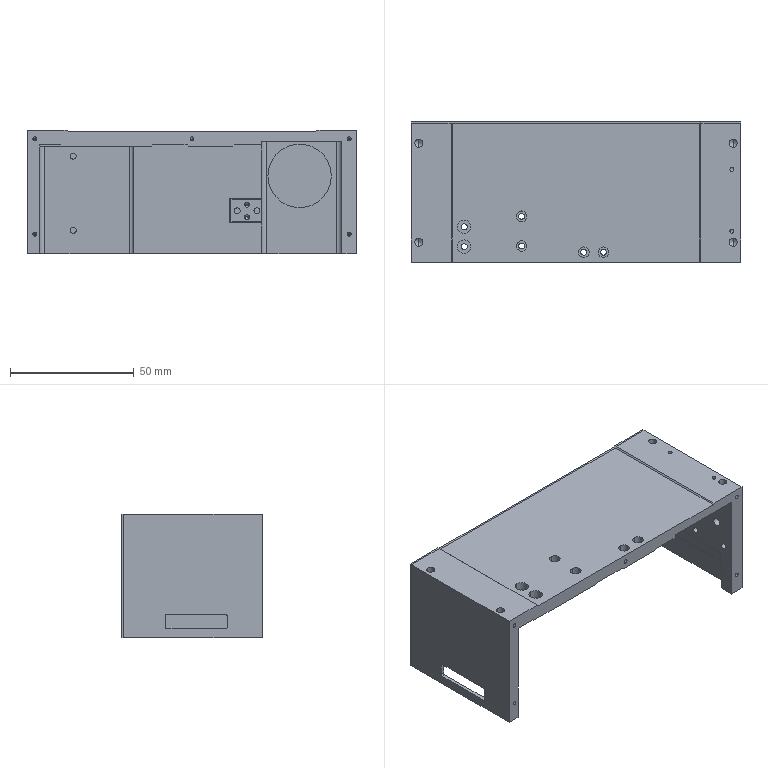NC program | NX | posted with a generic post | part box 133 x 56.74 x 50 mm
Whole program:
N10 G17 G21 G94 G90
(FLOOR_WALL_1_COPY , TOOL : D10)
N12 T10 M6
N14 G54
N16 G17 G0 G90 X22.033 Y-33. B0. C0. S9500 M3
N18 G43 Z30. H10
N20 Z2.685
N22 G94 G1 Z-0.315 F1000.
N24 Y-30.
N26 X-71.5 F2500.
N28 Y30.
N30 X-48.429
N32 X-47.929 Y29.5
N34 X47.929
N36 X48.429 Y30.
N38 X71.5
N40 Y-30.
N42 X22.033
N44 Y-25.
N46 X-66.5
N48 Y25.
N50 X-54.649
N52 G3 X-45.371 Y-15.019 R21.6
N54 G1 X-45.804 Y-20.
N56 X-61.5
N58 Y-13.085
N60 G3 X-45.804 Y-20. R26.6
N62 G1 X-45.371 Y-15.019
N64 G3 X-31.56 Y24.5 R21.6
N66 G1 X-32.113 Y23.667
N68 G2 X-26.333 Y-4.887 R20.6
N70 X-32.113 Y23.667 R-20.6
N72 G1 X-31.56 Y24.5
N74 X47.929
N76 G3 X50.108 Y25. R5.
N78 G1 X66.5
N80 Y-25.
N82 X22.033
N84 Y-20.
N86 X-41.196
N88 G3 X-20.293 Y19.5 R26.6
N90 G1 X47.929
N92 G3 X51.051 Y20. R10.
N94 G1 X61.5
N96 Y-20.
N98 X22.033
N100 Y-15.
N102 X-20.342
N104 G3 X-12.929 Y14.5 R31.6
N106 G1 X47.929
N108 G3 X51.77 Y15. R15.
N110 G1 X56.5
N112 Y-15.
N114 X22.033
N116 Y-10.
N118 X-10.83
N120 G3 X-7.023 Y9.5 R36.6
N122 G1 X47.929
N124 G3 X51.5 Y9.821 R20.
N126 G1 Y-10.
N128 X22.033
N130 Y-5.
N132 X-3.521
N134 G3 X-1.948 Y4.5 R41.6
N136 G1 X46.5
N138 Y-5.
N140 X22.033
N142 Y-0.5
N144 X2.065
N146 G3 X2.139 Y0. R46.1
N148 G1 X42.
N150 Y-0.5
N152 X22.033
N154 Y-3.5
N156 Z2.685
N158 G0 Z30.
N160 Y-33.
N162 Z2.36
N164 G1 Z-0.64 F1000.
N166 Y-30.
N168 X-71.5 F2500.
N170 Y30.
N172 X-48.429
N174 X-47.929 Y29.5
N176 X47.929
N178 X48.429 Y30.
N180 X71.5
N182 Y-30.
N184 X22.033
N186 Y-25.
N188 X-66.5
N190 Y25.
N192 X-54.649
N194 G3 X-45.371 Y-15.019 R21.6
N196 G1 X-45.804 Y-20.
N198 X-61.5
N200 Y-13.085
N202 G3 X-45.804 Y-20. R26.6
N204 G1 X-45.371 Y-15.019
N206 G3 X-31.56 Y24.5 R21.6
N208 G1 X-32.113 Y23.667
N210 G2 X-26.333 Y-4.887 R20.6
N212 X-32.113 Y23.667 R-20.6
N214 G1 X-31.56 Y24.5
N216 X47.929
N218 G3 X50.108 Y25. R5.
N220 G1 X66.5
N222 Y-25.
N224 X22.033
N226 Y-20.
N228 X-41.196
N230 G3 X-20.293 Y19.5 R26.6
N232 G1 X47.929
N234 G3 X51.051 Y20. R10.
N236 G1 X61.5
N238 Y-20.
N240 X22.033
N242 Y-15.
N244 X-20.342
N246 G3 X-12.929 Y14.5 R31.6
N248 G1 X47.929
N250 G3 X51.77 Y15. R15.
N252 G1 X56.5
N254 Y-15.
N256 X22.033
N258 Y-10.
N260 X-10.83
N262 G3 X-7.023 Y9.5 R36.6
N264 G1 X47.929
N266 G3 X51.5 Y9.821 R20.
N268 G1 Y-10.
N270 X22.033
N272 Y-5.
N274 X-3.521
N276 G3 X-1.948 Y4.5 R41.6
N278 G1 X46.5
N280 Y-5.
N282 X22.033
N284 Y-0.5
N286 X2.065
N288 G3 X2.139 Y0. R46.1
N290 G1 X42.
N292 Y-0.5
N294 X22.033
N296 Y-3.5
N298 Z2.36
N300 G0 Z30.
(HOLE_MILLING_1 , TOOL : D10)
N302 X-43.5 Y6.5
N304 Z1.
N306 G3 X-45.432 Y8.432 R1.932 F1650.
N308 X-47.364 Y6.5 R1.932
N310 X-47.364 Y6.5 Z0. I3.864 J0.
N312 X-47.364 Y6.5 Z-1. I3.864 J0.
N314 X-47.364 Y6.5 Z-2. I3.864 J0.
N316 X-47.364 Y6.5 Z-3. I3.864 J0.
N318 X-43.257 Y10.356 Z-3.74 R-3.864
N320 X-47.356 Y6.743 R3.864
N322 X-43.257 Y10.356 R-3.864
N324 X-45.307 Y8.549 R1.932
N326 X-43.5 Y6.5 R1.932
N328 G0 Z1.
N330 G3 X-47.364 Y10.364 R3.864
N332 X-51.228 Y6.5 R3.864
N334 X-51.228 Y6.5 Z0. I7.727 J0.
N336 X-51.228 Y6.5 Z-1. I7.727 J0.
N338 X-51.228 Y6.5 Z-2. I7.727 J0.
N340 X-51.228 Y6.5 Z-3. I7.727 J0.
N342 X-43.015 Y14.212 Z-3.74 R-7.727
N344 X-51.212 Y6.985 R7.727
N346 X-43.015 Y14.212 R-7.727
N348 X-47.114 Y10.599 R3.864
N350 X-43.5 Y6.5 R3.864
N352 G0 Z30.
N354 M5
(FLOOR_WALL_COPY_COPY , TOOL : D10JING)
N356 T09 M6
N358 G54
N360 G17 G0 G90 X-74.5 Y24.997 B0. C0. S9500 M3
N362 G43 Z30. H9
N364 Z2.26
N366 G94 G1 Z-0.74 F1250.
N368 X-71.5
N370 X-53.443
N372 G3 X-59.244 Y20.397 R21.
N374 G1 X-71.5
N376 Y15.798
N378 X-62.33
N380 G3 X-63.968 Y11.198 R21.
N382 G1 X-71.5
N384 Y6.598
N386 X-64.5
N388 G3 X-64.012 Y1.999 R21.
N390 G1 X-71.5
N392 Y-2.601
N394 X-62.425
N396 G3 X-59.415 Y-7.201 R21.
N398 G1 X-71.5
N400 Y-11.801
N402 X-53.8
N404 Z2.26
N406 G0 Z30.
N408 X-33.557 Y32.5
N410 Z2.26
N412 G1 Z-0.74
N414 Y24.997
N416 X71.5
N418 Y20.397
N420 X-27.756
N422 G2 X-24.67 Y15.798 R21.
N424 G1 X71.5
N426 Y11.198
N428 X-23.032
N430 G2 X-22.5 Y6.598 R21.
N432 G1 X71.5
N434 Y1.999
N436 X-22.988
N438 G2 X-24.575 Y-2.601 R21.
N440 G1 X71.5
N442 Y-7.201
N444 X-27.585
N446 G2 X-33.2 Y-11.801 R21.
N448 G1 X71.5
N450 Y-16.4
N452 X-71.5
N454 Y-21.
N456 X71.5
N458 X74.5
N460 Z2.26
N462 G0 Z30.
N464 X-43.5 Y32.5
N466 Z2.26
N468 G1 Z-0.74
N470 Y27.
N472 G2 X-23. Y6.5 R20.5
N474 X-43.5 Y27. R-20.5
N476 G1 Y30.5
N478 Z2.26
N480 G0 Z30.
(11_COPY , TOOL : D10JING)
N482 X-41.58 Y12.002
N484 Z-1.74
N486 G1 Z-3.74 F1000.
N488 X-42.634 Y13.828
N490 G3 X-43.5 Y14.328 R1.
N492 X-51.328 Y6.5 R7.827 F1200.
N494 X-43.5 Y14.328 R-7.827
N496 X-44.366 Y13.828 R1.
N498 G1 X-45.42 Y12.002
N500 Z-1.74
N502 G0 Z30.
N504 M5
(DRILLING_COPY_1_COPY_COPY_1_COPY , TOOL : D6A45)
N506 T07 M6
N508 G54
N510 G17 G0 G90 X-26.25 Y-7.64 B0. C0. S5000 M3
N512 G43 Z30. H7
N514 G94 G81 G98 Z-1.74 F250. R2.26
N516 X-18.25
N518 X48. Y-15.5
N520 Y14.5
N522 G80
N524 G0 X48. Y14.5 Z30.
N526 M5
(DRILLING_COPY_COPY_COPY_COPY_1 , TOOL : 2.4ZT)
N528 T12 M6
N530 G54
N532 G17 G0 G90 X-26.25 Y-7.64 B0. C0. S2000 M3
N534 G43 Z30. H12
N536 G94 G83 G98 Z-9.461 F150. Q2. R2.26
N538 X-18.25
N540 X48. Y-15.5 Z-7.961
N542 Y14.5
N544 G80
N546 G0 X48. Y14.5 Z30.
N548 M5
(HOLE_MILLING_COPY_1 , TOOL : D3)
N550 T03 M6
N552 G54
N554 G17 G0 G90 X-26.25 Y-7.64 B0. C0. S9500 M3
N556 G43 Z30. H3
N558 Z-0.24
N560 G94 G3 X-26.575 Y-7.315 R0.325 F1250.
N562 X-26.9 Y-7.64 R0.325
N564 X-26.9 Y-7.64 Z-0.49 I0.65 J0.
N566 X-26.9 Y-7.64 Z-0.74 I0.65 J0.
N568 X-26.9 Y-7.64 Z-0.99 I0.65 J0.
N570 X-26.9 Y-7.64 Z-1.24 I0.65 J0.
N572 X-26.9 Y-7.64 Z-1.49 I0.65 J0.
N574 X-26.9 Y-7.64 Z-1.74 I0.65 J0.
N576 X-26.9 Y-7.64 Z-1.99 I0.65 J0.
N578 X-26.9 Y-7.64 Z-2.24 I0.65 J0.
N580 X-26.9 Y-7.64 Z-2.49 I0.65 J0.
N582 X-26.9 Y-7.64 Z-2.74 I0.65 J0.
N584 X-26.9 Y-7.64 Z-2.99 I0.65 J0.
N586 X-26.451 Y-8.258 Z-3.04 R0.65
N588 X-25.632 Y-7.841 R0.65
N590 X-26.451 Y-8.258 R-0.65
N592 X-26.041 Y-8.05 R0.325
N594 X-26.25 Y-7.64 R0.325
N596 G0 Z30.
N598 X-18.25
N600 Z-0.24
N602 G3 X-18.575 Y-7.315 R0.325
N604 X-18.9 Y-7.64 R0.325
N606 X-18.9 Y-7.64 Z-0.49 I0.65 J0.
N608 X-18.9 Y-7.64 Z-0.74 I0.65 J0.
N610 X-18.9 Y-7.64 Z-0.99 I0.65 J0.
N612 X-18.9 Y-7.64 Z-1.24 I0.65 J0.
N614 X-18.9 Y-7.64 Z-1.49 I0.65 J0.
N616 X-18.9 Y-7.64 Z-1.74 I0.65 J0.
N618 X-18.9 Y-7.64 Z-1.99 I0.65 J0.
N620 X-18.9 Y-7.64 Z-2.24 I0.65 J0.
N622 X-18.9 Y-7.64 Z-2.49 I0.65 J0.
N624 X-18.9 Y-7.64 Z-2.74 I0.65 J0.
N626 X-18.9 Y-7.64 Z-2.99 I0.65 J0.
N628 X-18.451 Y-8.258 Z-3.04 R0.65
N630 X-17.632 Y-7.841 R0.65
N632 X-18.451 Y-8.258 R-0.65
N634 X-18.041 Y-8.05 R0.325
N636 X-18.25 Y-7.64 R0.325
N638 G0 Z30.
N640 X48. Y-15.5
N642 Z-0.24
N644 G3 X47.4 Y-14.9 R0.6
N646 X46.8 Y-15.5 R0.6
N648 X46.8 Y-15.5 Z-0.49 I1.2 J0.
N650 X46.8 Y-15.5 Z-0.74 I1.2 J0.
N652 X46.8 Y-15.5 Z-0.99 I1.2 J0.
N654 X46.8 Y-15.5 Z-1.24 I1.2 J0.
N656 X46.8 Y-15.5 Z-1.49 I1.2 J0.
N658 X46.8 Y-15.5 Z-1.74 I1.2 J0.
N660 X46.8 Y-15.5 Z-1.99 I1.2 J0.
N662 X46.8 Y-15.5 Z-2.24 I1.2 J0.
N664 X46.8 Y-15.5 Z-2.49 I1.2 J0.
N666 X46.8 Y-15.5 Z-2.74 I1.2 J0.
N668 X46.8 Y-15.5 Z-2.99 I1.2 J0.
N670 X46.8 Y-15.5 Z-3.24 I1.2 J0.
N672 X46.8 Y-15.5 Z-3.49 I1.2 J0.
N674 X46.8 Y-15.5 Z-3.74 I1.2 J0.
N676 X48. Y-16.7 R1.2
N678 X46.8 Y-15.5 R-1.2
N680 X47.4 Y-16.1 R0.6
N682 X48. Y-15.5 R0.6
N684 G0 Z30.
N686 Y14.5
N688 Z-0.24
N690 G3 X47.4 Y15.1 R0.6
N692 X46.8 Y14.5 R0.6
N694 X46.8 Y14.5 Z-0.49 I1.2 J0.
N696 X46.8 Y14.5 Z-0.74 I1.2 J0.
N698 X46.8 Y14.5 Z-0.99 I1.2 J0.
N700 X46.8 Y14.5 Z-1.24 I1.2 J0.
N702 X46.8 Y14.5 Z-1.49 I1.2 J0.
N704 X46.8 Y14.5 Z-1.74 I1.2 J0.
N706 X46.8 Y14.5 Z-1.99 I1.2 J0.
N708 X46.8 Y14.5 Z-2.24 I1.2 J0.
N710 X46.8 Y14.5 Z-2.49 I1.2 J0.
N712 X46.8 Y14.5 Z-2.74 I1.2 J0.
N714 X46.8 Y14.5 Z-2.99 I1.2 J0.
N716 X46.8 Y14.5 Z-3.24 I1.2 J0.
N718 X46.8 Y14.5 Z-3.49 I1.2 J0.
N720 X46.8 Y14.5 Z-3.74 I1.2 J0.
N722 X48. Y13.3 R1.2
N724 X46.8 Y14.5 R-1.2
N726 X47.4 Y13.9 R0.6
N728 X48. Y14.5 R0.6
N730 G0 Z30.
N732 M5
(PLANAR_MILL_COPY_1_COPY_COPY_COPY_COPY , TOOL : D6A45)
N734 T07 M6
N736 G54
N738 G17 G0 G90 X-32.854 Y5.183 B0. C0. S9500 M3
N740 G43 Z30. H7
N742 Z0.5
N744 G94 G1 Z-1. F1250.
N746 X-32.073 Y5.634
N748 G3 X-31.573 Y6.5 R1.
N750 X-43.5 Y18.428 R11.928
N752 X-31.573 Y6.5 R-11.928
N754 X-32.073 Y7.366 R1.
N756 G1 X-32.854 Y7.817
N758 Z0.5
N760 G0 Z30.
(PLANAR_MILL_COPY_1_COPY_COPY_COPY_COPY_COPY , TOOL : D6A45)
N762 X-27. Y-6.774
N764 Z-0.24
N766 G1 Z-1.74
N768 G3 X-27.5 Y-7.64 R1.
N770 X-26.25 Y-8.89 R1.25
N772 X-27.5 Y-7.64 R-1.25
N774 X-27. Y-8.506 R1.
N776 G1 Z-0.24
N778 G0 Z30.
N780 X-19. Y-6.774
N782 Z-0.24
N784 G1 Z-1.74
N786 G3 X-19.5 Y-7.64 R1.
N788 X-18.25 Y-8.89 R1.25
N790 X-19.5 Y-7.64 R-1.25
N792 X-19. Y-8.506 R1.
N794 G1 Z-0.24
N796 G0 Z30.
N798 X67.9 Y-24.134
N800 Z-0.24
N802 G1 Z-1.74
N804 G3 X67.4 Y-25. R1.
N806 G2 X66.5 Y-25.9 R0.9
N808 G1 X-66.5
N810 G2 X-67.4 Y-25. R0.9
N812 G1 Y25.
N814 G2 X-66.5 Y25.9 R0.9
N816 G1 X-50.5
N818 G2 X-49.864 Y25.636 R0.9
N820 G1 X-49.627 Y25.4
N822 X49.627
N824 X49.864 Y25.636
N826 G2 X50.5 Y25.9 R0.9
N828 G1 X66.5
N830 G2 X67.4 Y25. R0.9
N832 G1 Y-25.
N834 G3 X67.9 Y-25.866 R1.
N836 G1 Z-0.24
N838 G0 Z30.
N840 X46.7 Y15.366
N842 Z-0.24
N844 G1 Z-1.74
N846 G3 X46.2 Y14.5 R1.
N848 X48. Y12.7 R1.8
N850 X46.2 Y14.5 R-1.8
N852 X46.7 Y13.634 R1.
N854 G1 Z-0.24
N856 G0 Z30.
N858 Y-14.634
N860 Z-0.24
N862 G1 Z-1.74
N864 G3 X46.2 Y-15.5 R1.
N866 X48. Y-17.3 R1.8
N868 X46.2 Y-15.5 R-1.8
N870 X46.7 Y-16.366 R1.
N872 G1 Z-0.24
N874 G0 Z30.
N876 M5
N878 M2